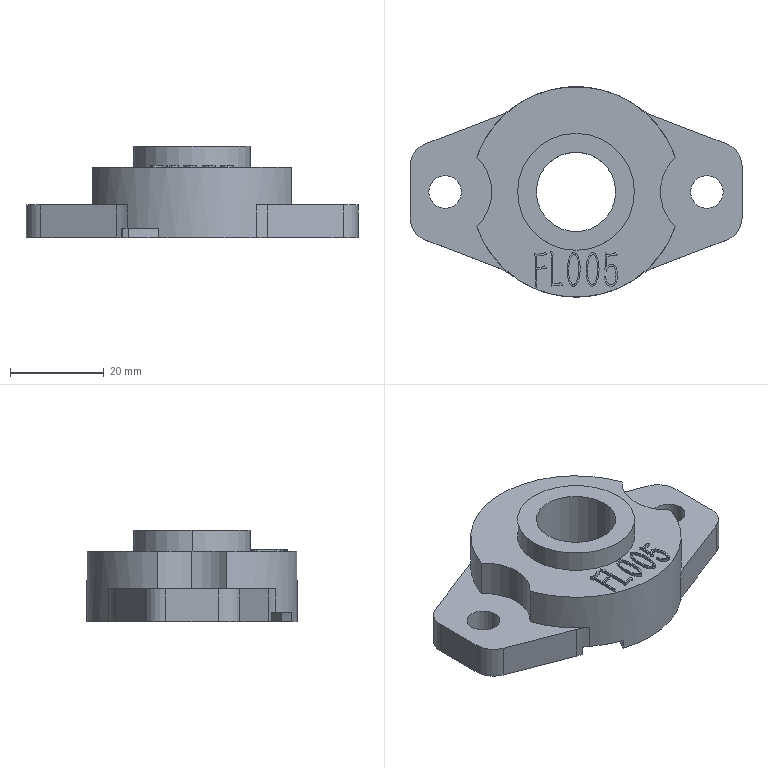Part | SolidWorks | features ICE 7, Fillet 2, MirrorPattern 2, Extrusion 1, HoleWzd 1, RefAxis 1 | 1 solid | 145 faces | box 71 x 45 x 19.5 mm | volume 23170 mm3 | plane 71 | spline 48 | cylinder 26 | commonest cylinder face diameters 20 x7 7 x4 10 x4 40 x3 9 x2 17 x2